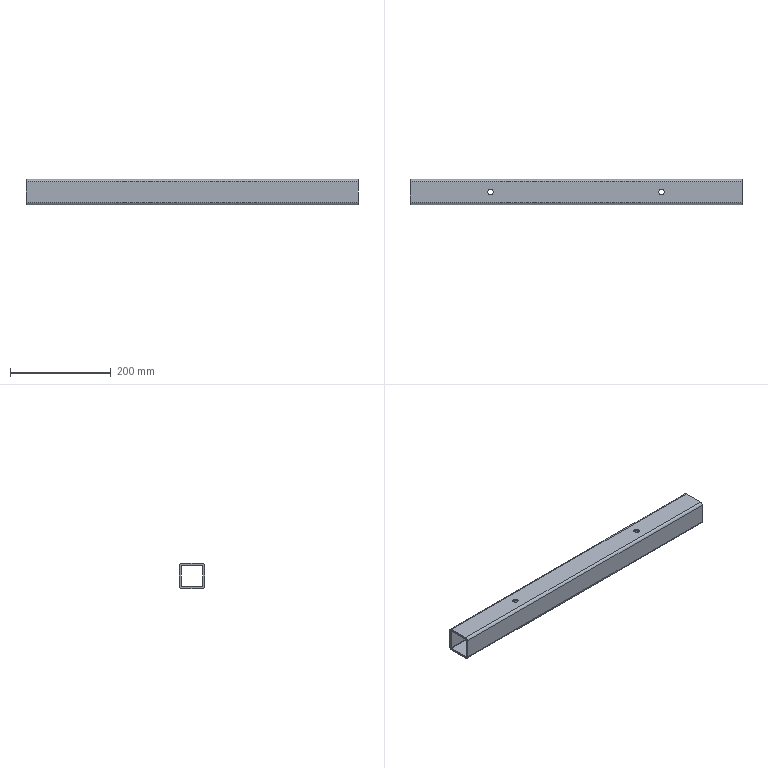Part | STEP file | 冲床-300配套压波_id1150_x_t | 1 solid | 22 faces | box 660 x 50 x 50 mm | volume 470724 mm3 | cylinder 12 | plane 10 | commonest cylinder face diameters 2 x4 10 x4 10.7 x4
STEP:
#1=CARTESIAN_POINT('',(1210.,275.,-66.));
#2=VERTEX_POINT('',#1);
#3=CARTESIAN_POINT('',(1210.,235.,-66.));
#4=VERTEX_POINT('',#3);
#5=CARTESIAN_POINT('',(1210.,30.,-66.));
#6=DIRECTION('',(0.,-1.,0.));
#7=VECTOR('',#6,1.);
#8=LINE('',#5,#7);
#9=EDGE_CURVE('',#2,#4,#8,.T.);
#10=ORIENTED_EDGE('',*,*,#9,.F.);
#11=CARTESIAN_POINT('',(1210.,276.,-65.));
#12=VERTEX_POINT('',#11);
#13=CARTESIAN_POINT('',(1210.,275.,-65.));
#14=DIRECTION('',(-1.,0.,0.));
#15=DIRECTION('',(0.,0.,1.));
#16=AXIS2_PLACEMENT_3D('',#13,#14,#15);
#17=CIRCLE('',#16,1.);
#18=EDGE_CURVE('',#12,#2,#17,.T.);
#19=ORIENTED_EDGE('',*,*,#18,.F.);
#20=CARTESIAN_POINT('',(1210.,276.,-25.));
#21=VERTEX_POINT('',#20);
#22=CARTESIAN_POINT('',(1210.,276.,-1220.));
#23=DIRECTION('',(0.,0.,-1.));
#24=VECTOR('',#23,1.);
#25=LINE('',#22,#24);
#26=EDGE_CURVE('',#21,#12,#25,.T.);
#27=ORIENTED_EDGE('',*,*,#26,.F.);
#28=CARTESIAN_POINT('',(1210.,275.,-24.));
#29=VERTEX_POINT('',#28);
#30=CARTESIAN_POINT('',(1210.,275.,-25.));
#31=DIRECTION('',(-1.,0.,0.));
#32=DIRECTION('',(0.,0.,1.));
#33=AXIS2_PLACEMENT_3D('',#30,#31,#32);
#34=CIRCLE('',#33,1.);
#35=EDGE_CURVE('',#29,#21,#34,.T.);
#36=ORIENTED_EDGE('',*,*,#35,.F.);
#37=CARTESIAN_POINT('',(1210.,235.,-24.));
#38=VERTEX_POINT('',#37);
#39=CARTESIAN_POINT('',(1210.,30.,-24.));
#40=DIRECTION('',(0.,1.,0.));
#41=VECTOR('',#40,1.);
#42=LINE('',#39,#41);
#43=EDGE_CURVE('',#38,#29,#42,.T.);
#44=ORIENTED_EDGE('',*,*,#43,.F.);
#45=CARTESIAN_POINT('',(1210.,234.,-25.));
#46=VERTEX_POINT('',#45);
#47=CARTESIAN_POINT('',(1210.,235.,-25.));
#48=DIRECTION('',(-1.,0.,0.));
#49=DIRECTION('',(0.,0.,1.));
#50=AXIS2_PLACEMENT_3D('',#47,#48,#49);
#51=CIRCLE('',#50,1.);
#52=EDGE_CURVE('',#46,#38,#51,.T.);
#53=ORIENTED_EDGE('',*,*,#52,.F.);
#54=CARTESIAN_POINT('',(1210.,234.,-65.));
#55=VERTEX_POINT('',#54);
#56=CARTESIAN_POINT('',(1210.,234.,-1220.));
#57=DIRECTION('',(0.,0.,1.));
#58=VECTOR('',#57,1.);
#59=LINE('',#56,#58);
#60=EDGE_CURVE('',#55,#46,#59,.T.);
#61=ORIENTED_EDGE('',*,*,#60,.F.);
#62=CARTESIAN_POINT('',(1210.,235.,-65.));
#63=DIRECTION('',(-1.,0.,0.));
#64=DIRECTION('',(0.,0.,1.));
#65=AXIS2_PLACEMENT_3D('',#62,#63,#64);
#66=CIRCLE('',#65,1.);
#67=EDGE_CURVE('',#4,#55,#66,.T.);
#68=ORIENTED_EDGE('',*,*,#67,.F.);
#69=EDGE_LOOP('',(#10,#19,#27,#36,#44,#53,#61,#68));
#70=FACE_BOUND('',#69,.T.);
#71=CARTESIAN_POINT('',(1210.,275.,-70.));
#72=VERTEX_POINT('',#71);
#73=CARTESIAN_POINT('',(1210.,235.,-70.));
#74=VERTEX_POINT('',#73);
#75=CARTESIAN_POINT('',(1210.,275.,-70.));
#76=DIRECTION('',(0.,-1.,0.));
#77=VECTOR('',#76,1.);
#78=LINE('',#75,#77);
#79=EDGE_CURVE('',#72,#74,#78,.T.);
#80=ORIENTED_EDGE('',*,*,#79,.T.);
#81=CARTESIAN_POINT('',(1210.,230.,-65.));
#82=VERTEX_POINT('',#81);
#83=CARTESIAN_POINT('',(1210.,235.,-65.));
#84=DIRECTION('',(-1.,0.,0.));
#85=DIRECTION('',(0.,0.,1.));
#86=AXIS2_PLACEMENT_3D('',#83,#84,#85);
#87=CIRCLE('',#86,5.);
#88=EDGE_CURVE('',#74,#82,#87,.T.);
#89=ORIENTED_EDGE('',*,*,#88,.T.);
#90=CARTESIAN_POINT('',(1210.,230.,-25.));
#91=VERTEX_POINT('',#90);
#92=CARTESIAN_POINT('',(1210.,230.,-65.));
#93=DIRECTION('',(0.,0.,1.));
#94=VECTOR('',#93,1.);
#95=LINE('',#92,#94);
#96=EDGE_CURVE('',#82,#91,#95,.T.);
#97=ORIENTED_EDGE('',*,*,#96,.T.);
#98=CARTESIAN_POINT('',(1210.,235.,-20.));
#99=VERTEX_POINT('',#98);
#100=CARTESIAN_POINT('',(1210.,235.,-25.));
#101=DIRECTION('',(-1.,0.,0.));
#102=DIRECTION('',(0.,0.,1.));
#103=AXIS2_PLACEMENT_3D('',#100,#101,#102);
#104=CIRCLE('',#103,5.);
#105=EDGE_CURVE('',#91,#99,#104,.T.);
#106=ORIENTED_EDGE('',*,*,#105,.T.);
#107=CARTESIAN_POINT('',(1210.,275.,-20.));
#108=VERTEX_POINT('',#107);
#109=CARTESIAN_POINT('',(1210.,235.,-20.));
#110=DIRECTION('',(0.,1.,0.));
#111=VECTOR('',#110,1.);
#112=LINE('',#109,#111);
#113=EDGE_CURVE('',#99,#108,#112,.T.);
#114=ORIENTED_EDGE('',*,*,#113,.T.);
#115=CARTESIAN_POINT('',(1210.,280.,-25.));
#116=VERTEX_POINT('',#115);
#117=CARTESIAN_POINT('',(1210.,275.,-25.));
#118=DIRECTION('',(-1.,0.,0.));
#119=DIRECTION('',(0.,0.,1.));
#120=AXIS2_PLACEMENT_3D('',#117,#118,#119);
#121=CIRCLE('',#120,5.);
#122=EDGE_CURVE('',#108,#116,#121,.T.);
#123=ORIENTED_EDGE('',*,*,#122,.T.);
#124=CARTESIAN_POINT('',(1210.,280.,-65.));
#125=VERTEX_POINT('',#124);
#126=CARTESIAN_POINT('',(1210.,280.,-25.));
#127=DIRECTION('',(0.,0.,-1.));
#128=VECTOR('',#127,1.);
#129=LINE('',#126,#128);
#130=EDGE_CURVE('',#116,#125,#129,.T.);
#131=ORIENTED_EDGE('',*,*,#130,.T.);
#132=CARTESIAN_POINT('',(1210.,275.,-65.));
#133=DIRECTION('',(-1.,0.,0.));
#134=DIRECTION('',(0.,0.,1.));
#135=AXIS2_PLACEMENT_3D('',#132,#133,#134);
#136=CIRCLE('',#135,5.);
#137=EDGE_CURVE('',#125,#72,#136,.T.);
#138=ORIENTED_EDGE('',*,*,#137,.T.);
#139=EDGE_LOOP('',(#80,#89,#97,#106,#114,#123,#131,#138));
#140=FACE_BOUND('',#139,.T.);
#141=CARTESIAN_POINT('',(1210.,30.,-1220.));
#142=DIRECTION('',(-1.,0.,0.));
#143=DIRECTION('',(0.,0.,1.));
#144=AXIS2_PLACEMENT_3D('',#141,#142,#143);
#145=PLANE('',#144);
#146=ADVANCED_FACE('',(#70,#140),#145,.T.);
#147=CARTESIAN_POINT('',(1870.,230.,-65.));
#148=VERTEX_POINT('',#147);
#149=CARTESIAN_POINT('',(1960.,230.,-65.));
#150=DIRECTION('',(-1.,0.,0.));
#151=VECTOR('',#150,1.);
#152=LINE('',#149,#151);
#153=EDGE_CURVE('',#148,#82,#152,.T.);
#154=ORIENTED_EDGE('',*,*,#153,.T.);
#155=ORIENTED_EDGE('',*,*,#88,.F.);
#156=CARTESIAN_POINT('',(1870.,235.,-70.));
#157=VERTEX_POINT('',#156);
#158=CARTESIAN_POINT('',(1960.,235.,-70.));
#159=DIRECTION('',(-1.,0.,0.));
#160=VECTOR('',#159,1.);
#161=LINE('',#158,#160);
#162=EDGE_CURVE('',#157,#74,#161,.T.);
#163=ORIENTED_EDGE('',*,*,#162,.F.);
#164=CARTESIAN_POINT('',(1870.,235.,-65.));
#165=DIRECTION('',(-1.,0.,0.));
#166=DIRECTION('',(0.,0.,1.));
#167=AXIS2_PLACEMENT_3D('',#164,#165,#166);
#168=CIRCLE('',#167,5.);
#169=EDGE_CURVE('',#157,#148,#168,.T.);
#170=ORIENTED_EDGE('',*,*,#169,.T.);
#171=EDGE_LOOP('',(#154,#155,#163,#170));
#172=FACE_OUTER_BOUND('',#171,.T.);
#173=CARTESIAN_POINT('',(1960.,235.,-65.));
#174=DIRECTION('',(-1.,0.,0.));
#175=DIRECTION('',(0.,0.,1.));
#176=AXIS2_PLACEMENT_3D('',#173,#174,#175);
#177=CYLINDRICAL_SURFACE('',#176,5.);
#178=ADVANCED_FACE('',(#172),#177,.T.);
#179=CARTESIAN_POINT('',(1870.,230.,-25.));
#180=VERTEX_POINT('',#179);
#181=CARTESIAN_POINT('',(1960.,230.,-25.));
#182=DIRECTION('',(-1.,0.,0.));
#183=VECTOR('',#182,1.);
#184=LINE('',#181,#183);
#185=EDGE_CURVE('',#180,#91,#184,.T.);
#186=ORIENTED_EDGE('',*,*,#185,.T.);
#187=ORIENTED_EDGE('',*,*,#96,.F.);
#188=ORIENTED_EDGE('',*,*,#153,.F.);
#189=CARTESIAN_POINT('',(1870.,230.,-740.));
#190=DIRECTION('',(0.,0.,1.));
#191=VECTOR('',#190,1.);
#192=LINE('',#189,#191);
#193=EDGE_CURVE('',#148,#180,#192,.T.);
#194=ORIENTED_EDGE('',*,*,#193,.T.);
#195=EDGE_LOOP('',(#186,#187,#188,#194));
#196=FACE_OUTER_BOUND('',#195,.T.);
#197=CARTESIAN_POINT('',(1960.,230.,-65.));
#198=DIRECTION('',(0.,-1.,0.));
#199=DIRECTION('',(0.,0.,1.));
#200=AXIS2_PLACEMENT_3D('',#197,#198,#199);
#201=PLANE('',#200);
#202=ADVANCED_FACE('',(#196),#201,.T.);
#203=CARTESIAN_POINT('',(1870.,235.,-20.));
#204=VERTEX_POINT('',#203);
#205=CARTESIAN_POINT('',(1960.,235.,-20.));
#206=DIRECTION('',(-1.,0.,0.));
#207=VECTOR('',#206,1.);
#208=LINE('',#205,#207);
#209=EDGE_CURVE('',#204,#99,#208,.T.);
#210=ORIENTED_EDGE('',*,*,#209,.T.);
#211=ORIENTED_EDGE('',*,*,#105,.F.);
#212=ORIENTED_EDGE('',*,*,#185,.F.);
#213=CARTESIAN_POINT('',(1870.,235.,-25.));
#214=DIRECTION('',(-1.,0.,0.));
#215=DIRECTION('',(0.,0.,1.));
#216=AXIS2_PLACEMENT_3D('',#213,#214,#215);
#217=CIRCLE('',#216,5.);
#218=EDGE_CURVE('',#180,#204,#217,.T.);
#219=ORIENTED_EDGE('',*,*,#218,.T.);
#220=EDGE_LOOP('',(#210,#211,#212,#219));
#221=FACE_OUTER_BOUND('',#220,.T.);
#222=CARTESIAN_POINT('',(1960.,235.,-25.));
#223=DIRECTION('',(-1.,0.,0.));
#224=DIRECTION('',(0.,0.,1.));
#225=AXIS2_PLACEMENT_3D('',#222,#223,#224);
#226=CYLINDRICAL_SURFACE('',#225,5.);
#227=ADVANCED_FACE('',(#221),#226,.T.);
#228=CARTESIAN_POINT('',(1375.35,255.,-20.));
#229=VERTEX_POINT('',#228);
#230=CARTESIAN_POINT('',(1370.,255.,-20.));
#231=DIRECTION('',(0.,0.,-1.));
#232=DIRECTION('',(1.,0.,0.));
#233=AXIS2_PLACEMENT_3D('',#230,#231,#232);
#234=CIRCLE('',#233,5.35);
#235=EDGE_CURVE('',#229,#229,#234,.T.);
#236=ORIENTED_EDGE('',*,*,#235,.T.);
#237=EDGE_LOOP('',(#236));
#238=FACE_BOUND('',#237,.T.);
#239=CARTESIAN_POINT('',(1715.35,255.,-20.));
#240=VERTEX_POINT('',#239);
#241=CARTESIAN_POINT('',(1710.,255.,-20.));
#242=DIRECTION('',(0.,0.,1.));
#243=DIRECTION('',(1.,0.,0.));
#244=AXIS2_PLACEMENT_3D('',#241,#242,#243);
#245=CIRCLE('',#244,5.35);
#246=EDGE_CURVE('',#240,#240,#245,.T.);
#247=ORIENTED_EDGE('',*,*,#246,.F.);
#248=EDGE_LOOP('',(#247));
#249=FACE_BOUND('',#248,.T.);
#250=CARTESIAN_POINT('',(1870.,275.,-20.));
#251=VERTEX_POINT('',#250);
#252=CARTESIAN_POINT('',(1960.,275.,-20.));
#253=DIRECTION('',(-1.,0.,0.));
#254=VECTOR('',#253,1.);
#255=LINE('',#252,#254);
#256=EDGE_CURVE('',#251,#108,#255,.T.);
#257=ORIENTED_EDGE('',*,*,#256,.T.);
#258=ORIENTED_EDGE('',*,*,#113,.F.);
#259=ORIENTED_EDGE('',*,*,#209,.F.);
#260=CARTESIAN_POINT('',(1870.,235.,-20.));
#261=DIRECTION('',(0.,1.,0.));
#262=VECTOR('',#261,1.);
#263=LINE('',#260,#262);
#264=EDGE_CURVE('',#204,#251,#263,.T.);
#265=ORIENTED_EDGE('',*,*,#264,.T.);
#266=EDGE_LOOP('',(#257,#258,#259,#265));
#267=FACE_BOUND('',#266,.T.);
#268=CARTESIAN_POINT('',(1960.,235.,-20.));
#269=DIRECTION('',(0.,0.,1.));
#270=DIRECTION('',(1.,0.,0.));
#271=AXIS2_PLACEMENT_3D('',#268,#269,#270);
#272=PLANE('',#271);
#273=ADVANCED_FACE('',(#238,#249,#267),#272,.T.);
#274=CARTESIAN_POINT('',(1870.,280.,-25.));
#275=VERTEX_POINT('',#274);
#276=CARTESIAN_POINT('',(1960.,280.,-25.));
#277=DIRECTION('',(-1.,0.,0.));
#278=VECTOR('',#277,1.);
#279=LINE('',#276,#278);
#280=EDGE_CURVE('',#275,#116,#279,.T.);
#281=ORIENTED_EDGE('',*,*,#280,.T.);
#282=ORIENTED_EDGE('',*,*,#122,.F.);
#283=ORIENTED_EDGE('',*,*,#256,.F.);
#284=CARTESIAN_POINT('',(1870.,275.,-25.));
#285=DIRECTION('',(-1.,0.,0.));
#286=DIRECTION('',(0.,0.,1.));
#287=AXIS2_PLACEMENT_3D('',#284,#285,#286);
#288=CIRCLE('',#287,5.);
#289=EDGE_CURVE('',#251,#275,#288,.T.);
#290=ORIENTED_EDGE('',*,*,#289,.T.);
#291=EDGE_LOOP('',(#281,#282,#283,#290));
#292=FACE_OUTER_BOUND('',#291,.T.);
#293=CARTESIAN_POINT('',(1960.,275.,-25.));
#294=DIRECTION('',(-1.,0.,0.));
#295=DIRECTION('',(0.,0.,1.));
#296=AXIS2_PLACEMENT_3D('',#293,#294,#295);
#297=CYLINDRICAL_SURFACE('',#296,5.);
#298=ADVANCED_FACE('',(#292),#297,.T.);
#299=CARTESIAN_POINT('',(1870.,276.,-65.));
#300=VERTEX_POINT('',#299);
#301=CARTESIAN_POINT('',(1870.,275.,-66.));
#302=VERTEX_POINT('',#301);
#303=CARTESIAN_POINT('',(1870.,275.,-65.));
#304=DIRECTION('',(-1.,0.,0.));
#305=DIRECTION('',(0.,0.,1.));
#306=AXIS2_PLACEMENT_3D('',#303,#304,#305);
#307=CIRCLE('',#306,1.);
#308=EDGE_CURVE('',#300,#302,#307,.T.);
#309=ORIENTED_EDGE('',*,*,#308,.T.);
#310=CARTESIAN_POINT('',(1870.,235.,-66.));
#311=VERTEX_POINT('',#310);
#312=CARTESIAN_POINT('',(1870.,235.,-66.));
#313=DIRECTION('',(0.,-1.,0.));
#314=VECTOR('',#313,1.);
#315=LINE('',#312,#314);
#316=EDGE_CURVE('',#302,#311,#315,.T.);
#317=ORIENTED_EDGE('',*,*,#316,.T.);
#318=CARTESIAN_POINT('',(1870.,234.,-65.));
#319=VERTEX_POINT('',#318);
#320=CARTESIAN_POINT('',(1870.,235.,-65.));
#321=DIRECTION('',(-1.,0.,0.));
#322=DIRECTION('',(0.,0.,1.));
#323=AXIS2_PLACEMENT_3D('',#320,#321,#322);
#324=CIRCLE('',#323,1.);
#325=EDGE_CURVE('',#311,#319,#324,.T.);
#326=ORIENTED_EDGE('',*,*,#325,.T.);
#327=CARTESIAN_POINT('',(1870.,234.,-25.));
#328=VERTEX_POINT('',#327);
#329=CARTESIAN_POINT('',(1870.,234.,-740.));
#330=DIRECTION('',(0.,0.,1.));
#331=VECTOR('',#330,1.);
#332=LINE('',#329,#331);
#333=EDGE_CURVE('',#319,#328,#332,.T.);
#334=ORIENTED_EDGE('',*,*,#333,.T.);
#335=CARTESIAN_POINT('',(1870.,235.,-24.));
#336=VERTEX_POINT('',#335);
#337=CARTESIAN_POINT('',(1870.,235.,-25.));
#338=DIRECTION('',(-1.,0.,0.));
#339=DIRECTION('',(0.,0.,1.));
#340=AXIS2_PLACEMENT_3D('',#337,#338,#339);
#341=CIRCLE('',#340,1.);
#342=EDGE_CURVE('',#328,#336,#341,.T.);
#343=ORIENTED_EDGE('',*,*,#342,.T.);
#344=CARTESIAN_POINT('',(1870.,275.,-24.));
#345=VERTEX_POINT('',#344);
#346=CARTESIAN_POINT('',(1870.,235.,-24.));
#347=DIRECTION('',(0.,1.,0.));
#348=VECTOR('',#347,1.);
#349=LINE('',#346,#348);
#350=EDGE_CURVE('',#336,#345,#349,.T.);
#351=ORIENTED_EDGE('',*,*,#350,.T.);
#352=CARTESIAN_POINT('',(1870.,276.,-25.));
#353=VERTEX_POINT('',#352);
#354=CARTESIAN_POINT('',(1870.,275.,-25.));
#355=DIRECTION('',(-1.,0.,0.));
#356=DIRECTION('',(0.,0.,1.));
#357=AXIS2_PLACEMENT_3D('',#354,#355,#356);
#358=CIRCLE('',#357,1.);
#359=EDGE_CURVE('',#345,#353,#358,.T.);
#360=ORIENTED_EDGE('',*,*,#359,.T.);
#361=CARTESIAN_POINT('',(1870.,276.,-740.));
#362=DIRECTION('',(0.,0.,-1.));
#363=VECTOR('',#362,1.);
#364=LINE('',#361,#363);
#365=EDGE_CURVE('',#353,#300,#364,.T.);
#366=ORIENTED_EDGE('',*,*,#365,.T.);
#367=EDGE_LOOP('',(#309,#317,#326,#334,#343,#351,#360,#366));
#368=FACE_BOUND('',#367,.T.);
#369=CARTESIAN_POINT('',(1870.,275.,-70.));
#370=VERTEX_POINT('',#369);
#371=CARTESIAN_POINT('',(1870.,235.,-70.));
#372=DIRECTION('',(0.,-1.,0.));
#373=VECTOR('',#372,1.);
#374=LINE('',#371,#373);
#375=EDGE_CURVE('',#370,#157,#374,.T.);
#376=ORIENTED_EDGE('',*,*,#375,.F.);
#377=CARTESIAN_POINT('',(1870.,280.,-65.));
#378=VERTEX_POINT('',#377);
#379=CARTESIAN_POINT('',(1870.,275.,-65.));
#380=DIRECTION('',(-1.,0.,0.));
#381=DIRECTION('',(0.,0.,1.));
#382=AXIS2_PLACEMENT_3D('',#379,#380,#381);
#383=CIRCLE('',#382,5.);
#384=EDGE_CURVE('',#378,#370,#383,.T.);
#385=ORIENTED_EDGE('',*,*,#384,.F.);
#386=CARTESIAN_POINT('',(1870.,280.,-740.));
#387=DIRECTION('',(0.,0.,-1.));
#388=VECTOR('',#387,1.);
#389=LINE('',#386,#388);
#390=EDGE_CURVE('',#275,#378,#389,.T.);
#391=ORIENTED_EDGE('',*,*,#390,.F.);
#392=ORIENTED_EDGE('',*,*,#289,.F.);
#393=ORIENTED_EDGE('',*,*,#264,.F.);
#394=ORIENTED_EDGE('',*,*,#218,.F.);
#395=ORIENTED_EDGE('',*,*,#193,.F.);
#396=ORIENTED_EDGE('',*,*,#169,.F.);
#397=EDGE_LOOP('',(#376,#385,#391,#392,#393,#394,#395,#396));
#398=FACE_BOUND('',#397,.T.);
#399=CARTESIAN_POINT('',(1870.,235.,-740.));
#400=DIRECTION('',(-1.,0.,0.));
#401=DIRECTION('',(0.,0.,-1.));
#402=AXIS2_PLACEMENT_3D('',#399,#400,#401);
#403=PLANE('',#402);
#404=ADVANCED_FACE('',(#368,#398),#403,.F.);
#405=CARTESIAN_POINT('',(1960.,280.,-65.));
#406=DIRECTION('',(-1.,0.,0.));
#407=VECTOR('',#406,1.);
#408=LINE('',#405,#407);
#409=EDGE_CURVE('',#378,#125,#408,.T.);
#410=ORIENTED_EDGE('',*,*,#409,.T.);
#411=ORIENTED_EDGE('',*,*,#130,.F.);
#412=ORIENTED_EDGE('',*,*,#280,.F.);
#413=ORIENTED_EDGE('',*,*,#390,.T.);
#414=EDGE_LOOP('',(#410,#411,#412,#413));
#415=FACE_OUTER_BOUND('',#414,.T.);
#416=CARTESIAN_POINT('',(1960.,280.,-25.));
#417=DIRECTION('',(0.,1.,0.));
#418=DIRECTION('',(0.,0.,-1.));
#419=AXIS2_PLACEMENT_3D('',#416,#417,#418);
#420=PLANE('',#419);
#421=ADVANCED_FACE('',(#415),#420,.T.);
#422=CARTESIAN_POINT('',(1364.65,255.,-70.));
#423=VERTEX_POINT('',#422);
#424=CARTESIAN_POINT('',(1370.,255.,-70.));
#425=DIRECTION('',(0.,0.,1.));
#426=DIRECTION('',(-1.,0.,0.));
#427=AXIS2_PLACEMENT_3D('',#424,#425,#426);
#428=CIRCLE('',#427,5.35);
#429=EDGE_CURVE('',#423,#423,#428,.T.);
#430=ORIENTED_EDGE('',*,*,#429,.T.);
#431=EDGE_LOOP('',(#430));
#432=FACE_BOUND('',#431,.T.);
#433=CARTESIAN_POINT('',(1704.65,255.,-70.));
#434=VERTEX_POINT('',#433);
#435=CARTESIAN_POINT('',(1710.,255.,-70.));
#436=DIRECTION('',(0.,0.,-1.));
#437=DIRECTION('',(-1.,0.,0.));
#438=AXIS2_PLACEMENT_3D('',#435,#436,#437);
#439=CIRCLE('',#438,5.35);
#440=EDGE_CURVE('',#434,#434,#439,.T.);
#441=ORIENTED_EDGE('',*,*,#440,.F.);
#442=EDGE_LOOP('',(#441));
#443=FACE_BOUND('',#442,.T.);
#444=ORIENTED_EDGE('',*,*,#162,.T.);
#445=ORIENTED_EDGE('',*,*,#79,.F.);
#446=CARTESIAN_POINT('',(1960.,275.,-70.));
#447=DIRECTION('',(-1.,0.,0.));
#448=VECTOR('',#447,1.);
#449=LINE('',#446,#448);
#450=EDGE_CURVE('',#370,#72,#449,.T.);
#451=ORIENTED_EDGE('',*,*,#450,.F.);
#452=ORIENTED_EDGE('',*,*,#375,.T.);
#453=EDGE_LOOP('',(#444,#445,#451,#452));
#454=FACE_BOUND('',#453,.T.);
#455=CARTESIAN_POINT('',(1960.,275.,-70.));
#456=DIRECTION('',(0.,0.,-1.));
#457=DIRECTION('',(-1.,0.,0.));
#458=AXIS2_PLACEMENT_3D('',#455,#456,#457);
#459=PLANE('',#458);
#460=ADVANCED_FACE('',(#432,#443,#454),#459,.T.);
#461=ORIENTED_EDGE('',*,*,#450,.T.);
#462=ORIENTED_EDGE('',*,*,#137,.F.);
#463=ORIENTED_EDGE('',*,*,#409,.F.);
#464=ORIENTED_EDGE('',*,*,#384,.T.);
#465=EDGE_LOOP('',(#461,#462,#463,#464));
#466=FACE_OUTER_BOUND('',#465,.T.);
#467=CARTESIAN_POINT('',(1960.,275.,-65.));
#468=DIRECTION('',(-1.,0.,0.));
#469=DIRECTION('',(0.,0.,1.));
#470=AXIS2_PLACEMENT_3D('',#467,#468,#469);
#471=CYLINDRICAL_SURFACE('',#470,5.);
#472=ADVANCED_FACE('',(#466),#471,.T.);
#473=CARTESIAN_POINT('',(1960.,234.,-65.));
#474=DIRECTION('',(-1.,0.,0.));
#475=VECTOR('',#474,1.);
#476=LINE('',#473,#475);
#477=EDGE_CURVE('',#319,#55,#476,.T.);
#478=ORIENTED_EDGE('',*,*,#477,.F.);
#479=ORIENTED_EDGE('',*,*,#325,.F.);
#480=CARTESIAN_POINT('',(1960.,235.,-66.));
#481=DIRECTION('',(-1.,0.,0.));
#482=VECTOR('',#481,1.);
#483=LINE('',#480,#482);
#484=EDGE_CURVE('',#311,#4,#483,.T.);
#485=ORIENTED_EDGE('',*,*,#484,.T.);
#486=ORIENTED_EDGE('',*,*,#67,.T.);
#487=EDGE_LOOP('',(#478,#479,#485,#486));
#488=FACE_OUTER_BOUND('',#487,.T.);
#489=CARTESIAN_POINT('',(1960.,235.,-65.));
#490=DIRECTION('',(-1.,0.,0.));
#491=DIRECTION('',(0.,0.,1.));
#492=AXIS2_PLACEMENT_3D('',#489,#490,#491);
#493=CYLINDRICAL_SURFACE('',#492,1.);
#494=ADVANCED_FACE('',(#488),#493,.F.);
#495=CARTESIAN_POINT('',(1960.,234.,-25.));
#496=DIRECTION('',(-1.,0.,0.));
#497=VECTOR('',#496,1.);
#498=LINE('',#495,#497);
#499=EDGE_CURVE('',#328,#46,#498,.T.);
#500=ORIENTED_EDGE('',*,*,#499,.F.);
#501=ORIENTED_EDGE('',*,*,#333,.F.);
#502=ORIENTED_EDGE('',*,*,#477,.T.);
#503=ORIENTED_EDGE('',*,*,#60,.T.);
#504=EDGE_LOOP('',(#500,#501,#502,#503));
#505=FACE_OUTER_BOUND('',#504,.T.);
#506=CARTESIAN_POINT('',(1960.,234.,-65.));
#507=DIRECTION('',(0.,-1.,0.));
#508=DIRECTION('',(0.,0.,1.));
#509=AXIS2_PLACEMENT_3D('',#506,#507,#508);
#510=PLANE('',#509);
#511=ADVANCED_FACE('',(#505),#510,.F.);
#512=CARTESIAN_POINT('',(1960.,235.,-24.));
#513=DIRECTION('',(-1.,0.,0.));
#514=VECTOR('',#513,1.);
#515=LINE('',#512,#514);
#516=EDGE_CURVE('',#336,#38,#515,.T.);
#517=ORIENTED_EDGE('',*,*,#516,.F.);
#518=ORIENTED_EDGE('',*,*,#342,.F.);
#519=ORIENTED_EDGE('',*,*,#499,.T.);
#520=ORIENTED_EDGE('',*,*,#52,.T.);
#521=EDGE_LOOP('',(#517,#518,#519,#520));
#522=FACE_OUTER_BOUND('',#521,.T.);
#523=CARTESIAN_POINT('',(1960.,235.,-25.));
#524=DIRECTION('',(-1.,0.,0.));
#525=DIRECTION('',(0.,0.,1.));
#526=AXIS2_PLACEMENT_3D('',#523,#524,#525);
#527=CYLINDRICAL_SURFACE('',#526,1.);
#528=ADVANCED_FACE('',(#522),#527,.F.);
#529=CARTESIAN_POINT('',(1375.35,255.,-24.));
#530=VERTEX_POINT('',#529);
#531=CARTESIAN_POINT('',(1370.,255.,-24.));
#532=DIRECTION('',(0.,0.,-1.));
#533=DIRECTION('',(1.,0.,0.));
#534=AXIS2_PLACEMENT_3D('',#531,#532,#533);
#535=CIRCLE('',#534,5.35);
#536=EDGE_CURVE('',#530,#530,#535,.T.);
#537=ORIENTED_EDGE('',*,*,#536,.F.);
#538=EDGE_LOOP('',(#537));
#539=FACE_BOUND('',#538,.T.);
#540=CARTESIAN_POINT('',(1715.35,255.,-24.));
#541=VERTEX_POINT('',#540);
#542=CARTESIAN_POINT('',(1710.,255.,-24.));
#543=DIRECTION('',(0.,0.,1.));
#544=DIRECTION('',(1.,0.,0.));
#545=AXIS2_PLACEMENT_3D('',#542,#543,#544);
#546=CIRCLE('',#545,5.35);
#547=EDGE_CURVE('',#541,#541,#546,.T.);
#548=ORIENTED_EDGE('',*,*,#547,.T.);
#549=EDGE_LOOP('',(#548));
#550=FACE_BOUND('',#549,.T.);
#551=CARTESIAN_POINT('',(1960.,275.,-24.));
#552=DIRECTION('',(-1.,0.,0.));
#553=VECTOR('',#552,1.);
#554=LINE('',#551,#553);
#555=EDGE_CURVE('',#345,#29,#554,.T.);
#556=ORIENTED_EDGE('',*,*,#555,.F.);
#557=ORIENTED_EDGE('',*,*,#350,.F.);
#558=ORIENTED_EDGE('',*,*,#516,.T.);
#559=ORIENTED_EDGE('',*,*,#43,.T.);
#560=EDGE_LOOP('',(#556,#557,#558,#559));
#561=FACE_BOUND('',#560,.T.);
#562=CARTESIAN_POINT('',(1960.,235.,-24.));
#563=DIRECTION('',(0.,0.,1.));
#564=DIRECTION('',(1.,0.,0.));
#565=AXIS2_PLACEMENT_3D('',#562,#563,#564);
#566=PLANE('',#565);
#567=ADVANCED_FACE('',(#539,#550,#561),#566,.F.);
#568=CARTESIAN_POINT('',(1960.,276.,-25.));
#569=DIRECTION('',(-1.,0.,0.));
#570=VECTOR('',#569,1.);
#571=LINE('',#568,#570);
#572=EDGE_CURVE('',#353,#21,#571,.T.);
#573=ORIENTED_EDGE('',*,*,#572,.F.);
#574=ORIENTED_EDGE('',*,*,#359,.F.);
#575=ORIENTED_EDGE('',*,*,#555,.T.);
#576=ORIENTED_EDGE('',*,*,#35,.T.);
#577=EDGE_LOOP('',(#573,#574,#575,#576));
#578=FACE_OUTER_BOUND('',#577,.T.);
#579=CARTESIAN_POINT('',(1960.,275.,-25.));
#580=DIRECTION('',(-1.,0.,0.));
#581=DIRECTION('',(0.,0.,1.));
#582=AXIS2_PLACEMENT_3D('',#579,#580,#581);
#583=CYLINDRICAL_SURFACE('',#582,1.);
#584=ADVANCED_FACE('',(#578),#583,.F.);
#585=CARTESIAN_POINT('',(1960.,276.,-65.));
#586=DIRECTION('',(-1.,0.,0.));
#587=VECTOR('',#586,1.);
#588=LINE('',#585,#587);
#589=EDGE_CURVE('',#300,#12,#588,.T.);
#590=ORIENTED_EDGE('',*,*,#589,.F.);
#591=ORIENTED_EDGE('',*,*,#365,.F.);
#592=ORIENTED_EDGE('',*,*,#572,.T.);
#593=ORIENTED_EDGE('',*,*,#26,.T.);
#594=EDGE_LOOP('',(#590,#591,#592,#593));
#595=FACE_OUTER_BOUND('',#594,.T.);
#596=CARTESIAN_POINT('',(1960.,276.,-25.));
#597=DIRECTION('',(0.,1.,0.));
#598=DIRECTION('',(0.,0.,-1.));
#599=AXIS2_PLACEMENT_3D('',#596,#597,#598);
#600=PLANE('',#599);
#601=ADVANCED_FACE('',(#595),#600,.F.);
#602=CARTESIAN_POINT('',(1364.65,255.,-66.));
#603=VERTEX_POINT('',#602);
#604=CARTESIAN_POINT('',(1370.,255.,-66.));
#605=DIRECTION('',(0.,0.,1.));
#606=DIRECTION('',(-1.,0.,0.));
#607=AXIS2_PLACEMENT_3D('',#604,#605,#606);
#608=CIRCLE('',#607,5.35);
#609=EDGE_CURVE('',#603,#603,#608,.T.);
#610=ORIENTED_EDGE('',*,*,#609,.F.);
#611=EDGE_LOOP('',(#610));
#612=FACE_BOUND('',#611,.T.);
#613=CARTESIAN_POINT('',(1704.65,255.,-66.));
#614=VERTEX_POINT('',#613);
#615=CARTESIAN_POINT('',(1710.,255.,-66.));
#616=DIRECTION('',(0.,0.,-1.));
#617=DIRECTION('',(-1.,0.,0.));
#618=AXIS2_PLACEMENT_3D('',#615,#616,#617);
#619=CIRCLE('',#618,5.35);
#620=EDGE_CURVE('',#614,#614,#619,.T.);
#621=ORIENTED_EDGE('',*,*,#620,.T.);
#622=EDGE_LOOP('',(#621));
#623=FACE_BOUND('',#622,.T.);
#624=ORIENTED_EDGE('',*,*,#484,.F.);
#625=ORIENTED_EDGE('',*,*,#316,.F.);
#626=CARTESIAN_POINT('',(1960.,275.,-66.));
#627=DIRECTION('',(-1.,0.,0.));
#628=VECTOR('',#627,1.);
#629=LINE('',#626,#628);
#630=EDGE_CURVE('',#302,#2,#629,.T.);
#631=ORIENTED_EDGE('',*,*,#630,.T.);
#632=ORIENTED_EDGE('',*,*,#9,.T.);
#633=EDGE_LOOP('',(#624,#625,#631,#632));
#634=FACE_BOUND('',#633,.T.);
#635=CARTESIAN_POINT('',(1960.,275.,-66.));
#636=DIRECTION('',(0.,0.,-1.));
#637=DIRECTION('',(-1.,0.,0.));
#638=AXIS2_PLACEMENT_3D('',#635,#636,#637);
#639=PLANE('',#638);
#640=ADVANCED_FACE('',(#612,#623,#634),#639,.F.);
#641=ORIENTED_EDGE('',*,*,#630,.F.);
#642=ORIENTED_EDGE('',*,*,#308,.F.);
#643=ORIENTED_EDGE('',*,*,#589,.T.);
#644=ORIENTED_EDGE('',*,*,#18,.T.);
#645=EDGE_LOOP('',(#641,#642,#643,#644));
#646=FACE_OUTER_BOUND('',#645,.T.);
#647=CARTESIAN_POINT('',(1960.,275.,-65.));
#648=DIRECTION('',(-1.,0.,0.));
#649=DIRECTION('',(0.,0.,1.));
#650=AXIS2_PLACEMENT_3D('',#647,#648,#649);
#651=CYLINDRICAL_SURFACE('',#650,1.);
#652=ADVANCED_FACE('',(#646),#651,.F.);
#653=ORIENTED_EDGE('',*,*,#440,.T.);
#654=EDGE_LOOP('',(#653));
#655=FACE_BOUND('',#654,.T.);
#656=ORIENTED_EDGE('',*,*,#620,.F.);
#657=EDGE_LOOP('',(#656));
#658=FACE_BOUND('',#657,.T.);
#659=CARTESIAN_POINT('',(1710.,255.,83.));
#660=DIRECTION('',(0.,0.,-1.));
#661=DIRECTION('',(-1.,0.,0.));
#662=AXIS2_PLACEMENT_3D('',#659,#660,#661);
#663=CYLINDRICAL_SURFACE('',#662,5.35);
#664=ADVANCED_FACE('',(#655,#658),#663,.F.);
#665=ORIENTED_EDGE('',*,*,#246,.T.);
#666=EDGE_LOOP('',(#665));
#667=FACE_BOUND('',#666,.T.);
#668=ORIENTED_EDGE('',*,*,#547,.F.);
#669=EDGE_LOOP('',(#668));
#670=FACE_BOUND('',#669,.T.);
#671=CARTESIAN_POINT('',(1710.,255.,83.));
#672=DIRECTION('',(0.,0.,-1.));
#673=DIRECTION('',(-1.,0.,0.));
#674=AXIS2_PLACEMENT_3D('',#671,#672,#673);
#675=CYLINDRICAL_SURFACE('',#674,5.35);
#676=ADVANCED_FACE('',(#667,#670),#675,.F.);
#677=ORIENTED_EDGE('',*,*,#429,.F.);
#678=EDGE_LOOP('',(#677));
#679=FACE_BOUND('',#678,.T.);
#680=ORIENTED_EDGE('',*,*,#609,.T.);
#681=EDGE_LOOP('',(#680));
#682=FACE_BOUND('',#681,.T.);
#683=CARTESIAN_POINT('',(1370.,255.,83.));
#684=DIRECTION('',(0.,0.,-1.));
#685=DIRECTION('',(-1.,0.,0.));
#686=AXIS2_PLACEMENT_3D('',#683,#684,#685);
#687=CYLINDRICAL_SURFACE('',#686,5.35);
#688=ADVANCED_FACE('',(#679,#682),#687,.F.);
#689=ORIENTED_EDGE('',*,*,#235,.F.);
#690=EDGE_LOOP('',(#689));
#691=FACE_BOUND('',#690,.T.);
#692=ORIENTED_EDGE('',*,*,#536,.T.);
#693=EDGE_LOOP('',(#692));
#694=FACE_BOUND('',#693,.T.);
#695=CARTESIAN_POINT('',(1370.,255.,83.));
#696=DIRECTION('',(0.,0.,-1.));
#697=DIRECTION('',(-1.,0.,0.));
#698=AXIS2_PLACEMENT_3D('',#695,#696,#697);
#699=CYLINDRICAL_SURFACE('',#698,5.35);
#700=ADVANCED_FACE('',(#691,#694),#699,.F.);
#701=CLOSED_SHELL('',(#146,#178,#202,#227,#273,#298,#404,#421,#460,#472,#494,#511,#528,#567,#584,#601,#640,#652,#664,#676,#688,#700));
#702=MANIFOLD_SOLID_BREP('',#701);
#703=(LENGTH_UNIT()NAMED_UNIT(*)SI_UNIT(.MILLI.,.METRE.));
#704=UNCERTAINTY_MEASURE_WITH_UNIT(LENGTH_MEASURE(0.00002),#703,'','');
#705=(NAMED_UNIT(*)PLANE_ANGLE_UNIT()SI_UNIT($,.RADIAN.));
#706=PLANE_ANGLE_MEASURE_WITH_UNIT(PLANE_ANGLE_MEASURE(0.01745),#705);
#707=DIMENSIONAL_EXPONENTS(0.,0.,0.,0.,0.,0.,0.);
#708=(CONVERSION_BASED_UNIT('DEGREE',#706)NAMED_UNIT(#707)PLANE_ANGLE_UNIT());
#709=(NAMED_UNIT(*)SI_UNIT($,.STERADIAN.)SOLID_ANGLE_UNIT());
#710=(GEOMETRIC_REPRESENTATION_CONTEXT(3)GLOBAL_UNCERTAINTY_ASSIGNED_CONTEXT((#704))GLOBAL_UNIT_ASSIGNED_CONTEXT((#703,#708,#709))REPRESENTATION_CONTEXT('',''));
#711=ADVANCED_BREP_SHAPE_REPRESENTATION('',(#702),#710);